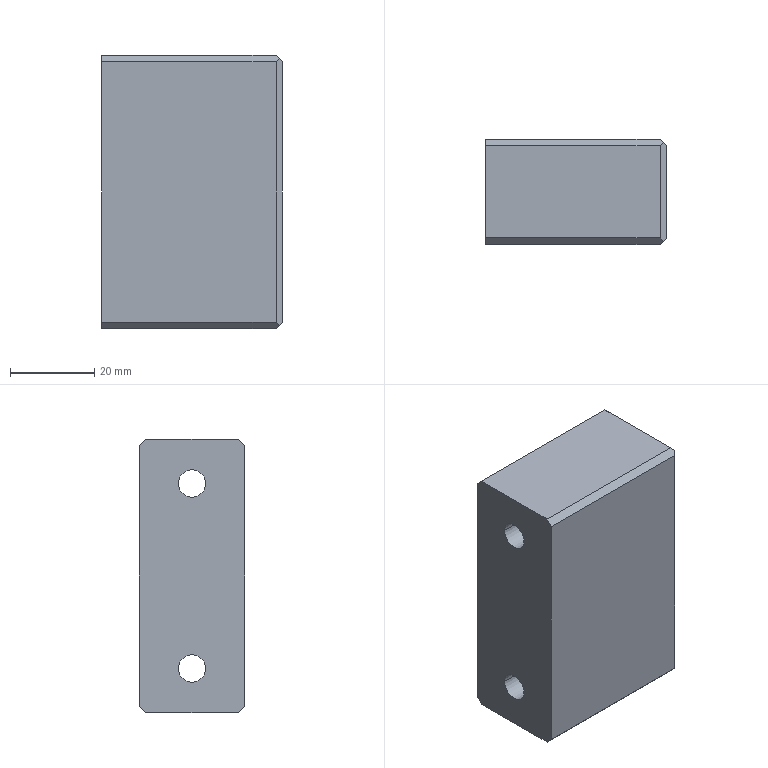Part | STEP file | SOLID | 1 solid | 34 faces | box 43 x 25 x 65 mm | volume 61003 mm3 | plane 16 | cylinder 10 | cone 8 | commonest cylinder face diameters 6.5 x4 11.5 x4 10.5 x2